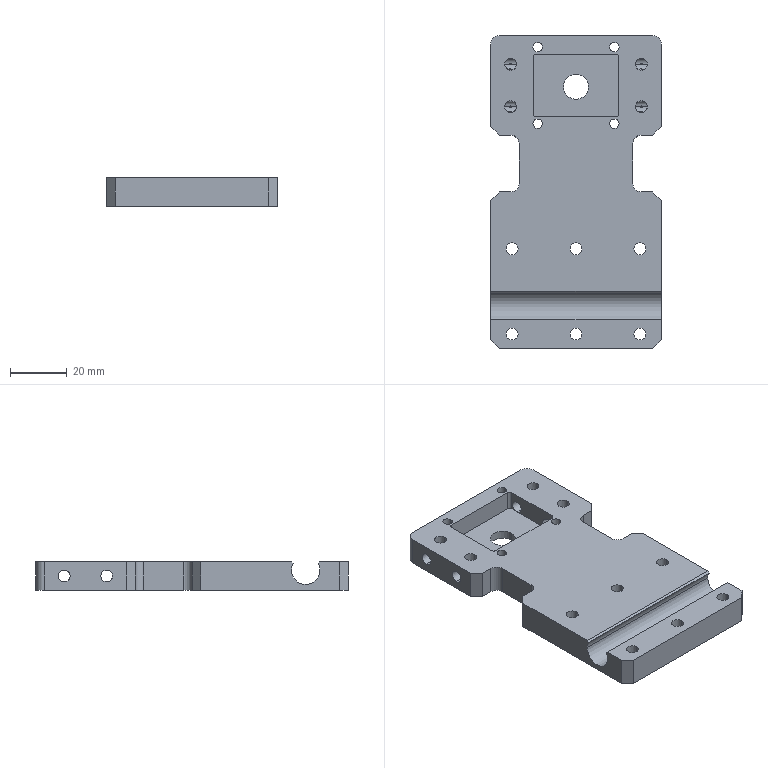Part | SolidWorks | features HoleWzd 5, Chamfer 2, Cut 2, Fillet 2, Extrusion 1, ICE 1, MirrorPattern 1 | 1 solid | 109 faces | box 60 x 110 x 10 mm | volume 50711 mm3 | cylinder 59 | plane 28 | cone 22 | commonest cylinder face diameters 4.2 x36 3.3 x8 6 x6 2 x4 10 x3 8.8 x2